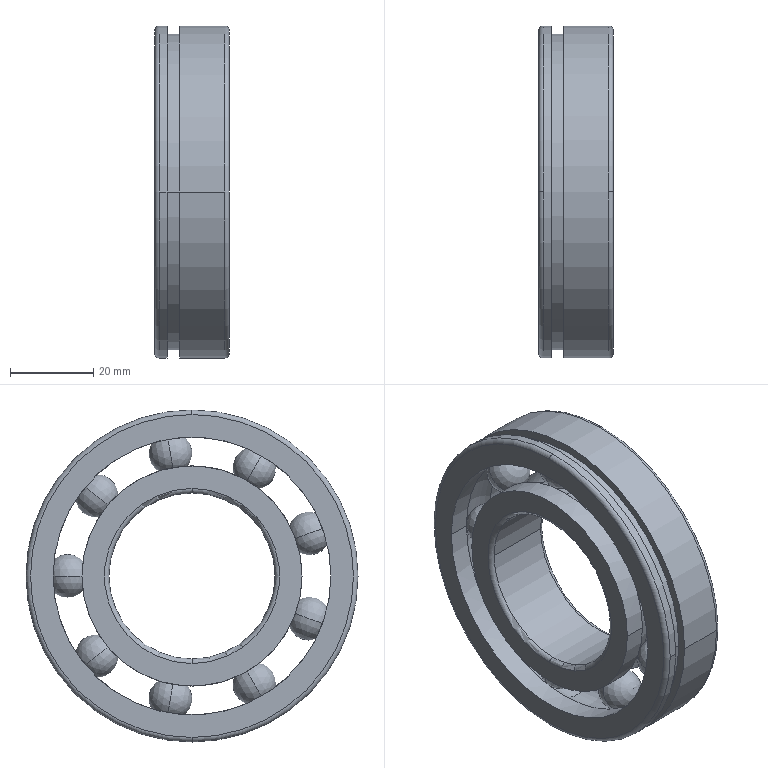Part | SolidWorks | features BaseBody 11 | 11 solids | 54 faces | box 18 x 80 x 80 mm | volume 44423 mm3 | sphere 18 | cylinder 16 | torus 14 | plane 6 | commonest cylinder face diameters 53.04 x4 66.96 x4 80 x4 40 x2 76.04 x2
STEP:
#1=CARTESIAN_POINT('',(9.,24.8,0.));
#2=VERTEX_POINT('',#1);
#3=CARTESIAN_POINT('',(9.,35.2,0.));
#4=VERTEX_POINT('',#3);
#5=CARTESIAN_POINT('',(9.,30.,0.));
#6=DIRECTION('',(0.,0.,1.));
#7=DIRECTION('',(1.,0.,0.));
#8=AXIS2_PLACEMENT_3D('',#5,#6,#7);
#9=CIRCLE('',#8,5.2);
#10=EDGE_CURVE('',#2,#4,#9,.T.);
#11=ORIENTED_EDGE('',*,*,#10,.F.);
#12=CARTESIAN_POINT('',(9.,30.,0.));
#13=DIRECTION('',(0.,0.,-1.));
#14=DIRECTION('',(-1.,0.,0.));
#15=AXIS2_PLACEMENT_3D('',#12,#13,#14);
#16=CIRCLE('',#15,5.2);
#17=EDGE_CURVE('',#2,#4,#16,.T.);
#18=ORIENTED_EDGE('',*,*,#17,.T.);
#19=EDGE_LOOP('',(#11,#18));
#20=FACE_OUTER_BOUND('',#19,.T.);
#21=CARTESIAN_POINT('',(9.,30.,0.));
#22=DIRECTION('',(0.,0.,-1.));
#23=DIRECTION('',(1.,0.,0.));
#24=AXIS2_PLACEMENT_3D('',#21,#22,#23);
#25=SPHERICAL_SURFACE('',#24,5.2);
#26=ADVANCED_FACE('',(#20),#25,.T.);
#27=ORIENTED_EDGE('',*,*,#17,.F.);
#28=ORIENTED_EDGE('',*,*,#10,.T.);
#29=EDGE_LOOP('',(#27,#28));
#30=FACE_OUTER_BOUND('',#29,.T.);
#31=CARTESIAN_POINT('',(9.,30.,0.));
#32=DIRECTION('',(0.,0.,-1.));
#33=DIRECTION('',(1.,0.,0.));
#34=AXIS2_PLACEMENT_3D('',#31,#32,#33);
#35=SPHERICAL_SURFACE('',#34,5.2);
#36=ADVANCED_FACE('',(#30),#35,.T.);
#37=CLOSED_SHELL('',(#26,#36));
#38=MANIFOLD_SOLID_BREP('',#37);
#39=CARTESIAN_POINT('',(6.,-38.02,0.));
#40=VERTEX_POINT('',#39);
#41=CARTESIAN_POINT('',(6.,38.02,0.));
#42=VERTEX_POINT('',#41);
#43=CARTESIAN_POINT('',(6.,0.,0.));
#44=DIRECTION('',(1.,0.,0.));
#45=DIRECTION('',(0.,1.,0.));
#46=AXIS2_PLACEMENT_3D('',#43,#44,#45);
#47=CIRCLE('',#46,38.02);
#48=EDGE_CURVE('',#40,#42,#47,.T.);
#49=ORIENTED_EDGE('',*,*,#48,.F.);
#50=CARTESIAN_POINT('',(3.,-38.02,0.));
#51=VERTEX_POINT('',#50);
#52=CARTESIAN_POINT('',(4.5,-38.02,0.));
#53=DIRECTION('',(-1.,0.,0.));
#54=VECTOR('',#53,1000.);
#55=LINE('',#52,#54);
#56=EDGE_CURVE('',#40,#51,#55,.T.);
#57=ORIENTED_EDGE('',*,*,#56,.T.);
#58=CARTESIAN_POINT('',(3.,38.02,0.));
#59=VERTEX_POINT('',#58);
#60=CARTESIAN_POINT('',(3.,0.,0.));
#61=DIRECTION('',(1.,0.,0.));
#62=DIRECTION('',(0.,1.,0.));
#63=AXIS2_PLACEMENT_3D('',#60,#61,#62);
#64=CIRCLE('',#63,38.02);
#65=EDGE_CURVE('',#51,#59,#64,.T.);
#66=ORIENTED_EDGE('',*,*,#65,.T.);
#67=CARTESIAN_POINT('',(4.5,38.02,0.));
#68=DIRECTION('',(-1.,0.,0.));
#69=VECTOR('',#68,1000.);
#70=LINE('',#67,#69);
#71=EDGE_CURVE('',#42,#59,#70,.T.);
#72=ORIENTED_EDGE('',*,*,#71,.F.);
#73=EDGE_LOOP('',(#49,#57,#66,#72));
#74=FACE_OUTER_BOUND('',#73,.T.);
#75=CARTESIAN_POINT('',(4.5,0.,0.));
#76=DIRECTION('',(-1.,0.,0.));
#77=DIRECTION('',(0.,1.,0.));
#78=AXIS2_PLACEMENT_3D('',#75,#76,#77);
#79=CYLINDRICAL_SURFACE('',#78,38.02);
#80=ADVANCED_FACE('',(#74),#79,.T.);
#81=CARTESIAN_POINT('',(16.9,-40.,0.));
#82=VERTEX_POINT('',#81);
#83=CARTESIAN_POINT('',(16.9,0.,-40.));
#84=VERTEX_POINT('',#83);
#85=CARTESIAN_POINT('',(16.9,0.,0.));
#86=DIRECTION('',(1.,0.,0.));
#87=DIRECTION('',(0.,-1.,0.));
#88=AXIS2_PLACEMENT_3D('',#85,#86,#87);
#89=CIRCLE('',#88,40.);
#90=EDGE_CURVE('',#82,#84,#89,.T.);
#91=ORIENTED_EDGE('',*,*,#90,.F.);
#92=CARTESIAN_POINT('',(6.,-40.,0.));
#93=VERTEX_POINT('',#92);
#94=CARTESIAN_POINT('',(12.,-40.,0.));
#95=DIRECTION('',(-1.,0.,0.));
#96=VECTOR('',#95,1000.);
#97=LINE('',#94,#96);
#98=EDGE_CURVE('',#82,#93,#97,.T.);
#99=ORIENTED_EDGE('',*,*,#98,.T.);
#100=CARTESIAN_POINT('',(6.,40.,0.));
#101=VERTEX_POINT('',#100);
#102=CARTESIAN_POINT('',(6.,0.,0.));
#103=DIRECTION('',(1.,0.,0.));
#104=DIRECTION('',(0.,1.,0.));
#105=AXIS2_PLACEMENT_3D('',#102,#103,#104);
#106=CIRCLE('',#105,40.);
#107=EDGE_CURVE('',#93,#101,#106,.T.);
#108=ORIENTED_EDGE('',*,*,#107,.T.);
#109=CARTESIAN_POINT('',(16.9,40.,0.));
#110=VERTEX_POINT('',#109);
#111=CARTESIAN_POINT('',(12.,40.,0.));
#112=DIRECTION('',(-1.,0.,0.));
#113=VECTOR('',#112,1000.);
#114=LINE('',#111,#113);
#115=EDGE_CURVE('',#110,#101,#114,.T.);
#116=ORIENTED_EDGE('',*,*,#115,.F.);
#117=CARTESIAN_POINT('',(16.9,0.,0.));
#118=DIRECTION('',(1.,0.,0.));
#119=DIRECTION('',(0.,-1.,0.));
#120=AXIS2_PLACEMENT_3D('',#117,#118,#119);
#121=CIRCLE('',#120,40.);
#122=EDGE_CURVE('',#84,#110,#121,.T.);
#123=ORIENTED_EDGE('',*,*,#122,.F.);
#124=EDGE_LOOP('',(#91,#99,#108,#116,#123));
#125=FACE_OUTER_BOUND('',#124,.T.);
#126=CARTESIAN_POINT('',(12.,0.,0.));
#127=DIRECTION('',(-1.,0.,0.));
#128=DIRECTION('',(0.,1.,0.));
#129=AXIS2_PLACEMENT_3D('',#126,#127,#128);
#130=CYLINDRICAL_SURFACE('',#129,40.);
#131=ADVANCED_FACE('',(#125),#130,.T.);
#132=CARTESIAN_POINT('',(3.,-40.,0.));
#133=VERTEX_POINT('',#132);
#134=CARTESIAN_POINT('',(3.,40.,0.));
#135=VERTEX_POINT('',#134);
#136=CARTESIAN_POINT('',(3.,0.,0.));
#137=DIRECTION('',(1.,0.,0.));
#138=DIRECTION('',(0.,1.,0.));
#139=AXIS2_PLACEMENT_3D('',#136,#137,#138);
#140=CIRCLE('',#139,40.);
#141=EDGE_CURVE('',#133,#135,#140,.T.);
#142=ORIENTED_EDGE('',*,*,#141,.F.);
#143=CARTESIAN_POINT('',(1.1,-40.,0.));
#144=VERTEX_POINT('',#143);
#145=CARTESIAN_POINT('',(1.5,-40.,0.));
#146=DIRECTION('',(-1.,0.,0.));
#147=VECTOR('',#146,1000.);
#148=LINE('',#145,#147);
#149=EDGE_CURVE('',#133,#144,#148,.T.);
#150=ORIENTED_EDGE('',*,*,#149,.T.);
#151=CARTESIAN_POINT('',(1.1,0.,-40.));
#152=VERTEX_POINT('',#151);
#153=CARTESIAN_POINT('',(1.1,0.,0.));
#154=DIRECTION('',(-1.,0.,0.));
#155=DIRECTION('',(0.,-1.,0.));
#156=AXIS2_PLACEMENT_3D('',#153,#154,#155);
#157=CIRCLE('',#156,40.);
#158=EDGE_CURVE('',#152,#144,#157,.T.);
#159=ORIENTED_EDGE('',*,*,#158,.F.);
#160=CARTESIAN_POINT('',(1.1,40.,0.));
#161=VERTEX_POINT('',#160);
#162=CARTESIAN_POINT('',(1.1,0.,0.));
#163=DIRECTION('',(-1.,0.,0.));
#164=DIRECTION('',(0.,-1.,0.));
#165=AXIS2_PLACEMENT_3D('',#162,#163,#164);
#166=CIRCLE('',#165,40.);
#167=EDGE_CURVE('',#161,#152,#166,.T.);
#168=ORIENTED_EDGE('',*,*,#167,.F.);
#169=CARTESIAN_POINT('',(1.5,40.,0.));
#170=DIRECTION('',(-1.,0.,0.));
#171=VECTOR('',#170,1000.);
#172=LINE('',#169,#171);
#173=EDGE_CURVE('',#135,#161,#172,.T.);
#174=ORIENTED_EDGE('',*,*,#173,.F.);
#175=EDGE_LOOP('',(#142,#150,#159,#168,#174));
#176=FACE_OUTER_BOUND('',#175,.T.);
#177=CARTESIAN_POINT('',(1.5,0.,0.));
#178=DIRECTION('',(-1.,0.,0.));
#179=DIRECTION('',(0.,1.,0.));
#180=AXIS2_PLACEMENT_3D('',#177,#178,#179);
#181=CYLINDRICAL_SURFACE('',#180,40.);
#182=ADVANCED_FACE('',(#176),#181,.T.);
#183=ORIENTED_EDGE('',*,*,#122,.T.);
#184=CARTESIAN_POINT('',(16.9,0.,40.));
#185=VERTEX_POINT('',#184);
#186=CARTESIAN_POINT('',(16.9,0.,0.));
#187=DIRECTION('',(1.,0.,0.));
#188=DIRECTION('',(0.,-1.,0.));
#189=AXIS2_PLACEMENT_3D('',#186,#187,#188);
#190=CIRCLE('',#189,40.);
#191=EDGE_CURVE('',#110,#185,#190,.T.);
#192=ORIENTED_EDGE('',*,*,#191,.T.);
#193=CARTESIAN_POINT('',(18.,0.,38.9));
#194=VERTEX_POINT('',#193);
#195=CARTESIAN_POINT('',(16.9,0.,38.9));
#196=DIRECTION('',(0.,1.,0.));
#197=DIRECTION('',(0.,0.,1.));
#198=AXIS2_PLACEMENT_3D('',#195,#196,#197);
#199=CIRCLE('',#198,1.1);
#200=EDGE_CURVE('',#185,#194,#199,.T.);
#201=ORIENTED_EDGE('',*,*,#200,.T.);
#202=CARTESIAN_POINT('',(18.,0.,-38.9));
#203=VERTEX_POINT('',#202);
#204=CARTESIAN_POINT('',(18.,0.,0.));
#205=DIRECTION('',(-1.,0.,0.));
#206=DIRECTION('',(0.,-1.,0.));
#207=AXIS2_PLACEMENT_3D('',#204,#205,#206);
#208=CIRCLE('',#207,38.9);
#209=EDGE_CURVE('',#194,#203,#208,.T.);
#210=ORIENTED_EDGE('',*,*,#209,.T.);
#211=CARTESIAN_POINT('',(16.9,0.,-38.9));
#212=DIRECTION('',(0.,-1.,0.));
#213=DIRECTION('',(0.,0.,-1.));
#214=AXIS2_PLACEMENT_3D('',#211,#212,#213);
#215=CIRCLE('',#214,1.1);
#216=EDGE_CURVE('',#84,#203,#215,.T.);
#217=ORIENTED_EDGE('',*,*,#216,.F.);
#218=EDGE_LOOP('',(#183,#192,#201,#210,#217));
#219=FACE_OUTER_BOUND('',#218,.T.);
#220=CARTESIAN_POINT('',(16.9,0.,0.));
#221=DIRECTION('',(1.,0.,0.));
#222=DIRECTION('',(0.,0.,-1.));
#223=AXIS2_PLACEMENT_3D('',#220,#221,#222);
#224=TOROIDAL_SURFACE('',#223,38.9,1.1);
#225=ADVANCED_FACE('',(#219),#224,.T.);
#226=CARTESIAN_POINT('',(0.,0.,-38.9));
#227=VERTEX_POINT('',#226);
#228=CARTESIAN_POINT('',(0.,0.,38.9));
#229=VERTEX_POINT('',#228);
#230=CARTESIAN_POINT('',(0.,0.,0.));
#231=DIRECTION('',(1.,0.,0.));
#232=DIRECTION('',(0.,-1.,0.));
#233=AXIS2_PLACEMENT_3D('',#230,#231,#232);
#234=CIRCLE('',#233,38.9);
#235=EDGE_CURVE('',#227,#229,#234,.T.);
#236=ORIENTED_EDGE('',*,*,#235,.T.);
#237=CARTESIAN_POINT('',(1.1,0.,40.));
#238=VERTEX_POINT('',#237);
#239=CARTESIAN_POINT('',(1.1,0.,38.9));
#240=DIRECTION('',(0.,1.,0.));
#241=DIRECTION('',(0.,0.,1.));
#242=AXIS2_PLACEMENT_3D('',#239,#240,#241);
#243=CIRCLE('',#242,1.1);
#244=EDGE_CURVE('',#229,#238,#243,.T.);
#245=ORIENTED_EDGE('',*,*,#244,.T.);
#246=CARTESIAN_POINT('',(1.1,0.,0.));
#247=DIRECTION('',(-1.,0.,0.));
#248=DIRECTION('',(0.,-1.,0.));
#249=AXIS2_PLACEMENT_3D('',#246,#247,#248);
#250=CIRCLE('',#249,40.);
#251=EDGE_CURVE('',#238,#161,#250,.T.);
#252=ORIENTED_EDGE('',*,*,#251,.T.);
#253=ORIENTED_EDGE('',*,*,#167,.T.);
#254=CARTESIAN_POINT('',(1.1,0.,-38.9));
#255=DIRECTION('',(0.,-1.,0.));
#256=DIRECTION('',(0.,0.,-1.));
#257=AXIS2_PLACEMENT_3D('',#254,#255,#256);
#258=CIRCLE('',#257,1.1);
#259=EDGE_CURVE('',#227,#152,#258,.T.);
#260=ORIENTED_EDGE('',*,*,#259,.F.);
#261=EDGE_LOOP('',(#236,#245,#252,#253,#260));
#262=FACE_OUTER_BOUND('',#261,.T.);
#263=CARTESIAN_POINT('',(1.1,0.,0.));
#264=DIRECTION('',(1.,0.,0.));
#265=DIRECTION('',(0.,0.,-1.));
#266=AXIS2_PLACEMENT_3D('',#263,#264,#265);
#267=TOROIDAL_SURFACE('',#266,38.9,1.1);
#268=ADVANCED_FACE('',(#262),#267,.T.);
#269=CARTESIAN_POINT('',(5.136,0.,33.48));
#270=VERTEX_POINT('',#269);
#271=CARTESIAN_POINT('',(5.136,-33.48,0.));
#272=VERTEX_POINT('',#271);
#273=CARTESIAN_POINT('',(5.136,0.,0.));
#274=DIRECTION('',(1.,0.,0.));
#275=DIRECTION('',(0.,1.,0.));
#276=AXIS2_PLACEMENT_3D('',#273,#274,#275);
#277=CIRCLE('',#276,33.48);
#278=EDGE_CURVE('',#270,#272,#277,.T.);
#279=ORIENTED_EDGE('',*,*,#278,.F.);
#280=CARTESIAN_POINT('',(12.864,0.,33.48));
#281=VERTEX_POINT('',#280);
#282=CARTESIAN_POINT('',(9.,0.,30.));
#283=DIRECTION('',(0.,1.,0.));
#284=DIRECTION('',(0.,0.,1.));
#285=AXIS2_PLACEMENT_3D('',#282,#283,#284);
#286=CIRCLE('',#285,5.2);
#287=EDGE_CURVE('',#270,#281,#286,.T.);
#288=ORIENTED_EDGE('',*,*,#287,.T.);
#289=CARTESIAN_POINT('',(12.864,-33.48,0.));
#290=VERTEX_POINT('',#289);
#291=CARTESIAN_POINT('',(12.864,0.,0.));
#292=DIRECTION('',(1.,0.,0.));
#293=DIRECTION('',(0.,1.,0.));
#294=AXIS2_PLACEMENT_3D('',#291,#292,#293);
#295=CIRCLE('',#294,33.48);
#296=EDGE_CURVE('',#281,#290,#295,.T.);
#297=ORIENTED_EDGE('',*,*,#296,.T.);
#298=CARTESIAN_POINT('',(12.864,0.,-33.48));
#299=VERTEX_POINT('',#298);
#300=CARTESIAN_POINT('',(12.864,0.,0.));
#301=DIRECTION('',(1.,0.,0.));
#302=DIRECTION('',(0.,1.,0.));
#303=AXIS2_PLACEMENT_3D('',#300,#301,#302);
#304=CIRCLE('',#303,33.48);
#305=EDGE_CURVE('',#290,#299,#304,.T.);
#306=ORIENTED_EDGE('',*,*,#305,.T.);
#307=CARTESIAN_POINT('',(5.136,0.,-33.48));
#308=VERTEX_POINT('',#307);
#309=CARTESIAN_POINT('',(9.,0.,-30.));
#310=DIRECTION('',(0.,-1.,0.));
#311=DIRECTION('',(0.,0.,-1.));
#312=AXIS2_PLACEMENT_3D('',#309,#310,#311);
#313=CIRCLE('',#312,5.2);
#314=EDGE_CURVE('',#308,#299,#313,.T.);
#315=ORIENTED_EDGE('',*,*,#314,.F.);
#316=CARTESIAN_POINT('',(5.136,0.,0.));
#317=DIRECTION('',(1.,0.,0.));
#318=DIRECTION('',(0.,1.,0.));
#319=AXIS2_PLACEMENT_3D('',#316,#317,#318);
#320=CIRCLE('',#319,33.48);
#321=EDGE_CURVE('',#272,#308,#320,.T.);
#322=ORIENTED_EDGE('',*,*,#321,.F.);
#323=EDGE_LOOP('',(#279,#288,#297,#306,#315,#322));
#324=FACE_OUTER_BOUND('',#323,.T.);
#325=CARTESIAN_POINT('',(9.,0.,0.));
#326=DIRECTION('',(1.,0.,0.));
#327=DIRECTION('',(0.,0.,-1.));
#328=AXIS2_PLACEMENT_3D('',#325,#326,#327);
#329=TOROIDAL_SURFACE('',#328,30.,5.2);
#330=ADVANCED_FACE('',(#324),#329,.F.);
#331=CARTESIAN_POINT('',(18.,33.48,0.));
#332=VERTEX_POINT('',#331);
#333=CARTESIAN_POINT('',(18.,-33.48,0.));
#334=VERTEX_POINT('',#333);
#335=CARTESIAN_POINT('',(18.,0.,0.));
#336=DIRECTION('',(1.,0.,0.));
#337=DIRECTION('',(0.,1.,0.));
#338=AXIS2_PLACEMENT_3D('',#335,#336,#337);
#339=CIRCLE('',#338,33.48);
#340=EDGE_CURVE('',#332,#334,#339,.T.);
#341=ORIENTED_EDGE('',*,*,#340,.T.);
#342=CARTESIAN_POINT('',(15.432,-33.48,0.));
#343=DIRECTION('',(-1.,0.,0.));
#344=VECTOR('',#343,1000.);
#345=LINE('',#342,#344);
#346=EDGE_CURVE('',#334,#290,#345,.T.);
#347=ORIENTED_EDGE('',*,*,#346,.T.);
#348=ORIENTED_EDGE('',*,*,#296,.F.);
#349=CARTESIAN_POINT('',(12.864,33.48,0.));
#350=VERTEX_POINT('',#349);
#351=CARTESIAN_POINT('',(12.864,0.,0.));
#352=DIRECTION('',(1.,0.,0.));
#353=DIRECTION('',(0.,1.,0.));
#354=AXIS2_PLACEMENT_3D('',#351,#352,#353);
#355=CIRCLE('',#354,33.48);
#356=EDGE_CURVE('',#350,#281,#355,.T.);
#357=ORIENTED_EDGE('',*,*,#356,.F.);
#358=CARTESIAN_POINT('',(15.432,33.48,0.));
#359=DIRECTION('',(-1.,0.,0.));
#360=VECTOR('',#359,1000.);
#361=LINE('',#358,#360);
#362=EDGE_CURVE('',#332,#350,#361,.T.);
#363=ORIENTED_EDGE('',*,*,#362,.F.);
#364=EDGE_LOOP('',(#341,#347,#348,#357,#363));
#365=FACE_OUTER_BOUND('',#364,.T.);
#366=CARTESIAN_POINT('',(15.432,0.,0.));
#367=DIRECTION('',(-1.,0.,0.));
#368=DIRECTION('',(0.,1.,0.));
#369=AXIS2_PLACEMENT_3D('',#366,#367,#368);
#370=CYLINDRICAL_SURFACE('',#369,33.48);
#371=ADVANCED_FACE('',(#365),#370,.F.);
#372=CARTESIAN_POINT('',(5.136,33.48,0.));
#373=VERTEX_POINT('',#372);
#374=CARTESIAN_POINT('',(5.136,0.,0.));
#375=DIRECTION('',(1.,0.,0.));
#376=DIRECTION('',(0.,1.,0.));
#377=AXIS2_PLACEMENT_3D('',#374,#375,#376);
#378=CIRCLE('',#377,33.48);
#379=EDGE_CURVE('',#373,#270,#378,.T.);
#380=ORIENTED_EDGE('',*,*,#379,.T.);
#381=ORIENTED_EDGE('',*,*,#278,.T.);
#382=CARTESIAN_POINT('',(0.,-33.48,0.));
#383=VERTEX_POINT('',#382);
#384=CARTESIAN_POINT('',(2.568,-33.48,0.));
#385=DIRECTION('',(-1.,0.,0.));
#386=VECTOR('',#385,1000.);
#387=LINE('',#384,#386);
#388=EDGE_CURVE('',#272,#383,#387,.T.);
#389=ORIENTED_EDGE('',*,*,#388,.T.);
#390=CARTESIAN_POINT('',(0.,33.48,0.));
#391=VERTEX_POINT('',#390);
#392=CARTESIAN_POINT('',(0.,0.,0.));
#393=DIRECTION('',(1.,0.,0.));
#394=DIRECTION('',(0.,1.,0.));
#395=AXIS2_PLACEMENT_3D('',#392,#393,#394);
#396=CIRCLE('',#395,33.48);
#397=EDGE_CURVE('',#391,#383,#396,.T.);
#398=ORIENTED_EDGE('',*,*,#397,.F.);
#399=CARTESIAN_POINT('',(2.568,33.48,0.));
#400=DIRECTION('',(-1.,0.,0.));
#401=VECTOR('',#400,1000.);
#402=LINE('',#399,#401);
#403=EDGE_CURVE('',#373,#391,#402,.T.);
#404=ORIENTED_EDGE('',*,*,#403,.F.);
#405=EDGE_LOOP('',(#380,#381,#389,#398,#404));
#406=FACE_OUTER_BOUND('',#405,.T.);
#407=CARTESIAN_POINT('',(2.568,0.,0.));
#408=DIRECTION('',(-1.,0.,0.));
#409=DIRECTION('',(0.,1.,0.));
#410=AXIS2_PLACEMENT_3D('',#407,#408,#409);
#411=CYLINDRICAL_SURFACE('',#410,33.48);
#412=ADVANCED_FACE('',(#406),#411,.F.);
#413=CARTESIAN_POINT('',(6.,0.,0.));
#414=DIRECTION('',(1.,0.,0.));
#415=DIRECTION('',(0.,1.,0.));
#416=AXIS2_PLACEMENT_3D('',#413,#414,#415);
#417=CIRCLE('',#416,38.02);
#418=EDGE_CURVE('',#42,#40,#417,.T.);
#419=ORIENTED_EDGE('',*,*,#418,.T.);
#420=ORIENTED_EDGE('',*,*,#48,.T.);
#421=EDGE_LOOP('',(#419,#420));
#422=FACE_BOUND('',#421,.T.);
#423=CARTESIAN_POINT('',(6.,0.,0.));
#424=DIRECTION('',(1.,0.,0.));
#425=DIRECTION('',(0.,1.,0.));
#426=AXIS2_PLACEMENT_3D('',#423,#424,#425);
#427=CIRCLE('',#426,40.);
#428=EDGE_CURVE('',#101,#93,#427,.T.);
#429=ORIENTED_EDGE('',*,*,#428,.F.);
#430=ORIENTED_EDGE('',*,*,#107,.F.);
#431=EDGE_LOOP('',(#429,#430));
#432=FACE_OUTER_BOUND('',#431,.T.);
#433=CARTESIAN_POINT('',(6.,39.01,0.));
#434=DIRECTION('',(-1.,0.,0.));
#435=DIRECTION('',(0.,0.,1.));
#436=AXIS2_PLACEMENT_3D('',#433,#434,#435);
#437=PLANE('',#436);
#438=ADVANCED_FACE('',(#422,#432),#437,.T.);
#439=CARTESIAN_POINT('',(3.,0.,0.));
#440=DIRECTION('',(1.,0.,0.));
#441=DIRECTION('',(0.,1.,0.));
#442=AXIS2_PLACEMENT_3D('',#439,#440,#441);
#443=CIRCLE('',#442,38.02);
#444=EDGE_CURVE('',#59,#51,#443,.T.);
#445=ORIENTED_EDGE('',*,*,#444,.F.);
#446=ORIENTED_EDGE('',*,*,#65,.F.);
#447=EDGE_LOOP('',(#445,#446));
#448=FACE_BOUND('',#447,.T.);
#449=CARTESIAN_POINT('',(3.,0.,0.));
#450=DIRECTION('',(1.,0.,0.));
#451=DIRECTION('',(0.,1.,0.));
#452=AXIS2_PLACEMENT_3D('',#449,#450,#451);
#453=CIRCLE('',#452,40.);
#454=EDGE_CURVE('',#135,#133,#453,.T.);
#455=ORIENTED_EDGE('',*,*,#454,.T.);
#456=ORIENTED_EDGE('',*,*,#141,.T.);
#457=EDGE_LOOP('',(#455,#456));
#458=FACE_OUTER_BOUND('',#457,.T.);
#459=CARTESIAN_POINT('',(3.,39.01,0.));
#460=DIRECTION('',(1.,0.,0.));
#461=DIRECTION('',(0.,1.,0.));
#462=AXIS2_PLACEMENT_3D('',#459,#460,#461);
#463=PLANE('',#462);
#464=ADVANCED_FACE('',(#448,#458),#463,.T.);
#465=ORIENTED_EDGE('',*,*,#340,.F.);
#466=CARTESIAN_POINT('',(18.,0.,0.));
#467=DIRECTION('',(1.,0.,0.));
#468=DIRECTION('',(0.,1.,0.));
#469=AXIS2_PLACEMENT_3D('',#466,#467,#468);
#470=CIRCLE('',#469,33.48);
#471=EDGE_CURVE('',#334,#332,#470,.T.);
#472=ORIENTED_EDGE('',*,*,#471,.F.);
#473=EDGE_LOOP('',(#465,#472));
#474=FACE_BOUND('',#473,.T.);
#475=CARTESIAN_POINT('',(18.,0.,0.));
#476=DIRECTION('',(-1.,0.,0.));
#477=DIRECTION('',(0.,-1.,0.));
#478=AXIS2_PLACEMENT_3D('',#475,#476,#477);
#479=CIRCLE('',#478,38.9);
#480=EDGE_CURVE('',#203,#194,#479,.T.);
#481=ORIENTED_EDGE('',*,*,#480,.F.);
#482=ORIENTED_EDGE('',*,*,#209,.F.);
#483=EDGE_LOOP('',(#481,#482));
#484=FACE_OUTER_BOUND('',#483,.T.);
#485=CARTESIAN_POINT('',(18.,36.74,0.));
#486=DIRECTION('',(1.,0.,0.));
#487=DIRECTION('',(0.,1.,0.));
#488=AXIS2_PLACEMENT_3D('',#485,#486,#487);
#489=PLANE('',#488);
#490=ADVANCED_FACE('',(#474,#484),#489,.T.);
#491=ORIENTED_EDGE('',*,*,#397,.T.);
#492=CARTESIAN_POINT('',(0.,0.,0.));
#493=DIRECTION('',(1.,0.,0.));
#494=DIRECTION('',(0.,1.,0.));
#495=AXIS2_PLACEMENT_3D('',#492,#493,#494);
#496=CIRCLE('',#495,33.48);
#497=EDGE_CURVE('',#383,#391,#496,.T.);
#498=ORIENTED_EDGE('',*,*,#497,.T.);
#499=EDGE_LOOP('',(#491,#498));
#500=FACE_BOUND('',#499,.T.);
#501=ORIENTED_EDGE('',*,*,#235,.F.);
#502=CARTESIAN_POINT('',(0.,0.,0.));
#503=DIRECTION('',(1.,0.,0.));
#504=DIRECTION('',(0.,-1.,0.));
#505=AXIS2_PLACEMENT_3D('',#502,#503,#504);
#506=CIRCLE('',#505,38.9);
#507=EDGE_CURVE('',#229,#227,#506,.T.);
#508=ORIENTED_EDGE('',*,*,#507,.F.);
#509=EDGE_LOOP('',(#501,#508));
#510=FACE_OUTER_BOUND('',#509,.T.);
#511=CARTESIAN_POINT('',(0.,36.74,0.));
#512=DIRECTION('',(-1.,0.,0.));
#513=DIRECTION('',(0.,0.,1.));
#514=AXIS2_PLACEMENT_3D('',#511,#512,#513);
#515=PLANE('',#514);
#516=ADVANCED_FACE('',(#500,#510),#515,.T.);
#517=ORIENTED_EDGE('',*,*,#388,.F.);
#518=ORIENTED_EDGE('',*,*,#321,.T.);
#519=CARTESIAN_POINT('',(5.136,0.,0.));
#520=DIRECTION('',(1.,0.,0.));
#521=DIRECTION('',(0.,1.,0.));
#522=AXIS2_PLACEMENT_3D('',#519,#520,#521);
#523=CIRCLE('',#522,33.48);
#524=EDGE_CURVE('',#308,#373,#523,.T.);
#525=ORIENTED_EDGE('',*,*,#524,.T.);
#526=ORIENTED_EDGE('',*,*,#403,.T.);
#527=ORIENTED_EDGE('',*,*,#497,.F.);
#528=EDGE_LOOP('',(#517,#518,#525,#526,#527));
#529=FACE_OUTER_BOUND('',#528,.T.);
#530=CARTESIAN_POINT('',(2.568,0.,0.));
#531=DIRECTION('',(-1.,0.,0.));
#532=DIRECTION('',(0.,1.,0.));
#533=AXIS2_PLACEMENT_3D('',#530,#531,#532);
#534=CYLINDRICAL_SURFACE('',#533,33.48);
#535=ADVANCED_FACE('',(#529),#534,.F.);
#536=ORIENTED_EDGE('',*,*,#346,.F.);
#537=ORIENTED_EDGE('',*,*,#471,.T.);
#538=ORIENTED_EDGE('',*,*,#362,.T.);
#539=CARTESIAN_POINT('',(12.864,0.,0.));
#540=DIRECTION('',(1.,0.,0.));
#541=DIRECTION('',(0.,1.,0.));
#542=AXIS2_PLACEMENT_3D('',#539,#540,#541);
#543=CIRCLE('',#542,33.48);
#544=EDGE_CURVE('',#299,#350,#543,.T.);
#545=ORIENTED_EDGE('',*,*,#544,.F.);
#546=ORIENTED_EDGE('',*,*,#305,.F.);
#547=EDGE_LOOP('',(#536,#537,#538,#545,#546));
#548=FACE_OUTER_BOUND('',#547,.T.);
#549=CARTESIAN_POINT('',(15.432,0.,0.));
#550=DIRECTION('',(-1.,0.,0.));
#551=DIRECTION('',(0.,1.,0.));
#552=AXIS2_PLACEMENT_3D('',#549,#550,#551);
#553=CYLINDRICAL_SURFACE('',#552,33.48);
#554=ADVANCED_FACE('',(#548),#553,.F.);
#555=ORIENTED_EDGE('',*,*,#287,.F.);
#556=ORIENTED_EDGE('',*,*,#379,.F.);
#557=ORIENTED_EDGE('',*,*,#524,.F.);
#558=ORIENTED_EDGE('',*,*,#314,.T.);
#559=ORIENTED_EDGE('',*,*,#544,.T.);
#560=ORIENTED_EDGE('',*,*,#356,.T.);
#561=EDGE_LOOP('',(#555,#556,#557,#558,#559,#560));
#562=FACE_OUTER_BOUND('',#561,.T.);
#563=CARTESIAN_POINT('',(9.,0.,0.));
#564=DIRECTION('',(1.,0.,0.));
#565=DIRECTION('',(0.,0.,-1.));
#566=AXIS2_PLACEMENT_3D('',#563,#564,#565);
#567=TOROIDAL_SURFACE('',#566,30.,5.2);
#568=ADVANCED_FACE('',(#562),#567,.F.);
#569=ORIENTED_EDGE('',*,*,#244,.F.);
#570=ORIENTED_EDGE('',*,*,#507,.T.);
#571=ORIENTED_EDGE('',*,*,#259,.T.);
#572=ORIENTED_EDGE('',*,*,#158,.T.);
#573=CARTESIAN_POINT('',(1.1,0.,0.));
#574=DIRECTION('',(-1.,0.,0.));
#575=DIRECTION('',(0.,-1.,0.));
#576=AXIS2_PLACEMENT_3D('',#573,#574,#575);
#577=CIRCLE('',#576,40.);
#578=EDGE_CURVE('',#144,#238,#577,.T.);
#579=ORIENTED_EDGE('',*,*,#578,.T.);
#580=EDGE_LOOP('',(#569,#570,#571,#572,#579));
#581=FACE_OUTER_BOUND('',#580,.T.);
#582=CARTESIAN_POINT('',(1.1,0.,0.));
#583=DIRECTION('',(1.,0.,0.));
#584=DIRECTION('',(0.,0.,-1.));
#585=AXIS2_PLACEMENT_3D('',#582,#583,#584);
#586=TOROIDAL_SURFACE('',#585,38.9,1.1);
#587=ADVANCED_FACE('',(#581),#586,.T.);
#588=ORIENTED_EDGE('',*,*,#200,.F.);
#589=CARTESIAN_POINT('',(16.9,0.,0.));
#590=DIRECTION('',(1.,0.,0.));
#591=DIRECTION('',(0.,-1.,0.));
#592=AXIS2_PLACEMENT_3D('',#589,#590,#591);
#593=CIRCLE('',#592,40.);
#594=EDGE_CURVE('',#185,#82,#593,.T.);
#595=ORIENTED_EDGE('',*,*,#594,.T.);
#596=ORIENTED_EDGE('',*,*,#90,.T.);
#597=ORIENTED_EDGE('',*,*,#216,.T.);
#598=ORIENTED_EDGE('',*,*,#480,.T.);
#599=EDGE_LOOP('',(#588,#595,#596,#597,#598));
#600=FACE_OUTER_BOUND('',#599,.T.);
#601=CARTESIAN_POINT('',(16.9,0.,0.));
#602=DIRECTION('',(1.,0.,0.));
#603=DIRECTION('',(0.,0.,-1.));
#604=AXIS2_PLACEMENT_3D('',#601,#602,#603);
#605=TOROIDAL_SURFACE('',#604,38.9,1.1);
#606=ADVANCED_FACE('',(#600),#605,.T.);
#607=ORIENTED_EDGE('',*,*,#149,.F.);
#608=ORIENTED_EDGE('',*,*,#454,.F.);
#609=ORIENTED_EDGE('',*,*,#173,.T.);
#610=ORIENTED_EDGE('',*,*,#251,.F.);
#611=ORIENTED_EDGE('',*,*,#578,.F.);
#612=EDGE_LOOP('',(#607,#608,#609,#610,#611));
#613=FACE_OUTER_BOUND('',#612,.T.);
#614=CARTESIAN_POINT('',(1.5,0.,0.));
#615=DIRECTION('',(-1.,0.,0.));
#616=DIRECTION('',(0.,1.,0.));
#617=AXIS2_PLACEMENT_3D('',#614,#615,#616);
#618=CYLINDRICAL_SURFACE('',#617,40.);
#619=ADVANCED_FACE('',(#613),#618,.T.);
#620=ORIENTED_EDGE('',*,*,#98,.F.);
#621=ORIENTED_EDGE('',*,*,#594,.F.);
#622=ORIENTED_EDGE('',*,*,#191,.F.);
#623=ORIENTED_EDGE('',*,*,#115,.T.);
#624=ORIENTED_EDGE('',*,*,#428,.T.);
#625=EDGE_LOOP('',(#620,#621,#622,#623,#624));
#626=FACE_OUTER_BOUND('',#625,.T.);
#627=CARTESIAN_POINT('',(12.,0.,0.));
#628=DIRECTION('',(-1.,0.,0.));
#629=DIRECTION('',(0.,1.,0.));
#630=AXIS2_PLACEMENT_3D('',#627,#628,#629);
#631=CYLINDRICAL_SURFACE('',#630,40.);
#632=ADVANCED_FACE('',(#626),#631,.T.);
#633=ORIENTED_EDGE('',*,*,#56,.F.);
#634=ORIENTED_EDGE('',*,*,#418,.F.);
#635=ORIENTED_EDGE('',*,*,#71,.T.);
#636=ORIENTED_EDGE('',*,*,#444,.T.);
#637=EDGE_LOOP('',(#633,#634,#635,#636));
#638=FACE_OUTER_BOUND('',#637,.T.);
#639=CARTESIAN_POINT('',(4.5,0.,0.));
#640=DIRECTION('',(-1.,0.,0.));
#641=DIRECTION('',(0.,1.,0.));
#642=AXIS2_PLACEMENT_3D('',#639,#640,#641);
#643=CYLINDRICAL_SURFACE('',#642,38.02);
#644=ADVANCED_FACE('',(#638),#643,.T.);
#645=CLOSED_SHELL('',(#80,#131,#182,#225,#268,#330,#371,#412,#438,#464,#490,#516,#535,#554,#568,#587,#606,#619,#632,#644));
#646=MANIFOLD_SOLID_BREP('',#645);
#647=CARTESIAN_POINT('',(12.864,0.,-26.52));
#648=VERTEX_POINT('',#647);
#649=CARTESIAN_POINT('',(9.,0.,-24.8));
#650=VERTEX_POINT('',#649);
#651=CARTESIAN_POINT('',(9.,0.,-30.));
#652=DIRECTION('',(0.,-1.,0.));
#653=DIRECTION('',(0.,0.,-1.));
#654=AXIS2_PLACEMENT_3D('',#651,#652,#653);
#655=CIRCLE('',#654,5.2);
#656=EDGE_CURVE('',#648,#650,#655,.T.);
#657=ORIENTED_EDGE('',*,*,#656,.T.);
#658=CARTESIAN_POINT('',(9.,0.,24.8));
#659=VERTEX_POINT('',#658);
#660=CARTESIAN_POINT('',(9.,0.,0.));
#661=DIRECTION('',(1.,0.,0.));
#662=DIRECTION('',(0.,0.,-1.));
#663=AXIS2_PLACEMENT_3D('',#660,#661,#662);
#664=CIRCLE('',#663,24.8);
#665=EDGE_CURVE('',#650,#659,#664,.T.);
#666=ORIENTED_EDGE('',*,*,#665,.T.);
#667=CARTESIAN_POINT('',(12.864,0.,26.52));
#668=VERTEX_POINT('',#667);
#669=CARTESIAN_POINT('',(9.,0.,30.));
#670=DIRECTION('',(0.,1.,0.));
#671=DIRECTION('',(0.,0.,1.));
#672=AXIS2_PLACEMENT_3D('',#669,#670,#671);
#673=CIRCLE('',#672,5.2);
#674=EDGE_CURVE('',#668,#659,#673,.T.);
#675=ORIENTED_EDGE('',*,*,#674,.F.);
#676=CARTESIAN_POINT('',(12.864,26.52,0.));
#677=VERTEX_POINT('',#676);
#678=CARTESIAN_POINT('',(12.864,0.,0.));
#679=DIRECTION('',(1.,0.,0.));
#680=DIRECTION('',(0.,1.,0.));
#681=AXIS2_PLACEMENT_3D('',#678,#679,#680);
#682=CIRCLE('',#681,26.52);
#683=EDGE_CURVE('',#677,#668,#682,.T.);
#684=ORIENTED_EDGE('',*,*,#683,.F.);
#685=CARTESIAN_POINT('',(12.864,0.,0.));
#686=DIRECTION('',(1.,0.,0.));
#687=DIRECTION('',(0.,1.,0.));
#688=AXIS2_PLACEMENT_3D('',#685,#686,#687);
#689=CIRCLE('',#688,26.52);
#690=EDGE_CURVE('',#648,#677,#689,.T.);
#691=ORIENTED_EDGE('',*,*,#690,.F.);
#692=EDGE_LOOP('',(#657,#666,#675,#684,#691));
#693=FACE_OUTER_BOUND('',#692,.T.);
#694=CARTESIAN_POINT('',(9.,0.,0.));
#695=DIRECTION('',(1.,0.,0.));
#696=DIRECTION('',(0.,0.,-1.));
#697=AXIS2_PLACEMENT_3D('',#694,#695,#696);
#698=TOROIDAL_SURFACE('',#697,30.,5.2);
#699=ADVANCED_FACE('',(#693),#698,.F.);
#700=ORIENTED_EDGE('',*,*,#674,.T.);
#701=CARTESIAN_POINT('',(9.,0.,0.));
#702=DIRECTION('',(1.,0.,0.));
#703=DIRECTION('',(0.,0.,-1.));
#704=AXIS2_PLACEMENT_3D('',#701,#702,#703);
#705=CIRCLE('',#704,24.8);
#706=EDGE_CURVE('',#659,#650,#705,.T.);
#707=ORIENTED_EDGE('',*,*,#706,.T.);
#708=ORIENTED_EDGE('',*,*,#656,.F.);
#709=CARTESIAN_POINT('',(12.864,-26.52,0.));
#710=VERTEX_POINT('',#709);
#711=CARTESIAN_POINT('',(12.864,0.,0.));
#712=DIRECTION('',(1.,0.,0.));
#713=DIRECTION('',(0.,1.,0.));
#714=AXIS2_PLACEMENT_3D('',#711,#712,#713);
#715=CIRCLE('',#714,26.52);
#716=EDGE_CURVE('',#710,#648,#715,.T.);
#717=ORIENTED_EDGE('',*,*,#716,.F.);
#718=CARTESIAN_POINT('',(12.864,0.,0.));
#719=DIRECTION('',(1.,0.,0.));
#720=DIRECTION('',(0.,1.,0.));
#721=AXIS2_PLACEMENT_3D('',#718,#719,#720);
#722=CIRCLE('',#721,26.52);
#723=EDGE_CURVE('',#668,#710,#722,.T.);
#724=ORIENTED_EDGE('',*,*,#723,.F.);
#725=EDGE_LOOP('',(#700,#707,#708,#717,#724));
#726=FACE_OUTER_BOUND('',#725,.T.);
#727=CARTESIAN_POINT('',(9.,0.,0.));
#728=DIRECTION('',(1.,0.,0.));
#729=DIRECTION('',(0.,0.,-1.));
#730=AXIS2_PLACEMENT_3D('',#727,#728,#729);
#731=TOROIDAL_SURFACE('',#730,30.,5.2);
#732=ADVANCED_FACE('',(#726),#731,.F.);
#733=ORIENTED_EDGE('',*,*,#706,.F.);
#734=CARTESIAN_POINT('',(5.136,0.,26.52));
#735=VERTEX_POINT('',#734);
#736=CARTESIAN_POINT('',(9.,0.,30.));
#737=DIRECTION('',(0.,1.,0.));
#738=DIRECTION('',(0.,0.,1.));
#739=AXIS2_PLACEMENT_3D('',#736,#737,#738);
#740=CIRCLE('',#739,5.2);
#741=EDGE_CURVE('',#659,#735,#740,.T.);
#742=ORIENTED_EDGE('',*,*,#741,.T.);
#743=CARTESIAN_POINT('',(5.136,-26.52,0.));
#744=VERTEX_POINT('',#743);
#745=CARTESIAN_POINT('',(5.136,0.,0.));
#746=DIRECTION('',(1.,0.,0.));
#747=DIRECTION('',(0.,1.,0.));
#748=AXIS2_PLACEMENT_3D('',#745,#746,#747);
#749=CIRCLE('',#748,26.52);
#750=EDGE_CURVE('',#735,#744,#749,.T.);
#751=ORIENTED_EDGE('',*,*,#750,.T.);
#752=CARTESIAN_POINT('',(5.136,0.,-26.52));
#753=VERTEX_POINT('',#752);
#754=CARTESIAN_POINT('',(5.136,0.,0.));
#755=DIRECTION('',(1.,0.,0.));
#756=DIRECTION('',(0.,1.,0.));
#757=AXIS2_PLACEMENT_3D('',#754,#755,#756);
#758=CIRCLE('',#757,26.52);
#759=EDGE_CURVE('',#744,#753,#758,.T.);
#760=ORIENTED_EDGE('',*,*,#759,.T.);
#761=CARTESIAN_POINT('',(9.,0.,-30.));
#762=DIRECTION('',(0.,-1.,0.));
#763=DIRECTION('',(0.,0.,-1.));
#764=AXIS2_PLACEMENT_3D('',#761,#762,#763);
#765=CIRCLE('',#764,5.2);
#766=EDGE_CURVE('',#650,#753,#765,.T.);
#767=ORIENTED_EDGE('',*,*,#766,.F.);
#768=EDGE_LOOP('',(#733,#742,#751,#760,#767));
#769=FACE_OUTER_BOUND('',#768,.T.);
#770=CARTESIAN_POINT('',(9.,0.,0.));
#771=DIRECTION('',(1.,0.,0.));
#772=DIRECTION('',(0.,0.,-1.));
#773=AXIS2_PLACEMENT_3D('',#770,#771,#772);
#774=TOROIDAL_SURFACE('',#773,30.,5.2);
#775=ADVANCED_FACE('',(#769),#774,.F.);
#776=CARTESIAN_POINT('',(16.9,-20.,0.));
#777=VERTEX_POINT('',#776);
#778=CARTESIAN_POINT('',(16.9,0.,20.));
#779=VERTEX_POINT('',#778);
#780=CARTESIAN_POINT('',(16.9,0.,0.));
#781=DIRECTION('',(-1.,0.,0.));
#782=DIRECTION('',(0.,-1.,0.));
#783=AXIS2_PLACEMENT_3D('',#780,#781,#782);
#784=CIRCLE('',#783,20.);
#785=EDGE_CURVE('',#777,#779,#784,.T.);
#786=ORIENTED_EDGE('',*,*,#785,.F.);
#787=CARTESIAN_POINT('',(1.1,-20.,0.));
#788=VERTEX_POINT('',#787);
#789=CARTESIAN_POINT('',(9.,-20.,0.));
#790=DIRECTION('',(-1.,0.,0.));
#791=VECTOR('',#790,1000.);
#792=LINE('',#789,#791);
#793=EDGE_CURVE('',#777,#788,#792,.T.);
#794=ORIENTED_EDGE('',*,*,#793,.T.);
#795=CARTESIAN_POINT('',(1.1,0.,20.));
#796=VERTEX_POINT('',#795);
#797=CARTESIAN_POINT('',(1.1,0.,0.));
#798=DIRECTION('',(1.,0.,0.));
#799=DIRECTION('',(0.,-1.,0.));
#800=AXIS2_PLACEMENT_3D('',#797,#798,#799);
#801=CIRCLE('',#800,20.);
#802=EDGE_CURVE('',#796,#788,#801,.T.);
#803=ORIENTED_EDGE('',*,*,#802,.F.);
#804=CARTESIAN_POINT('',(1.1,20.,0.));
#805=VERTEX_POINT('',#804);
#806=CARTESIAN_POINT('',(1.1,0.,0.));
#807=DIRECTION('',(1.,0.,0.));
#808=DIRECTION('',(0.,-1.,0.));
#809=AXIS2_PLACEMENT_3D('',#806,#807,#808);
#810=CIRCLE('',#809,20.);
#811=EDGE_CURVE('',#805,#796,#810,.T.);
#812=ORIENTED_EDGE('',*,*,#811,.F.);
#813=CARTESIAN_POINT('',(16.9,20.,0.));
#814=VERTEX_POINT('',#813);
#815=CARTESIAN_POINT('',(9.,20.,0.));
#816=DIRECTION('',(-1.,0.,0.));
#817=VECTOR('',#816,1000.);
#818=LINE('',#815,#817);
#819=EDGE_CURVE('',#814,#805,#818,.T.);
#820=ORIENTED_EDGE('',*,*,#819,.F.);
#821=CARTESIAN_POINT('',(16.9,0.,0.));
#822=DIRECTION('',(-1.,0.,0.));
#823=DIRECTION('',(0.,-1.,0.));
#824=AXIS2_PLACEMENT_3D('',#821,#822,#823);
#825=CIRCLE('',#824,20.);
#826=EDGE_CURVE('',#779,#814,#825,.T.);
#827=ORIENTED_EDGE('',*,*,#826,.F.);
#828=EDGE_LOOP('',(#786,#794,#803,#812,#820,#827));
#829=FACE_OUTER_BOUND('',#828,.T.);
#830=CARTESIAN_POINT('',(9.,0.,0.));
#831=DIRECTION('',(-1.,0.,0.));
#832=DIRECTION('',(0.,1.,0.));
#833=AXIS2_PLACEMENT_3D('',#830,#831,#832);
#834=CYLINDRICAL_SURFACE('',#833,20.);
#835=ADVANCED_FACE('',(#829),#834,.F.);
#836=CARTESIAN_POINT('',(1.1,0.,-20.));
#837=VERTEX_POINT('',#836);
#838=CARTESIAN_POINT('',(1.1,0.,0.));
#839=DIRECTION('',(1.,0.,0.));
#840=DIRECTION('',(0.,-1.,0.));
#841=AXIS2_PLACEMENT_3D('',#838,#839,#840);
#842=CIRCLE('',#841,20.);
#843=EDGE_CURVE('',#837,#805,#842,.T.);
#844=ORIENTED_EDGE('',*,*,#843,.T.);
#845=ORIENTED_EDGE('',*,*,#811,.T.);
#846=CARTESIAN_POINT('',(0.,0.,21.1));
#847=VERTEX_POINT('',#846);
#848=CARTESIAN_POINT('',(1.1,0.,21.1));
#849=DIRECTION('',(0.,1.,0.));
#850=DIRECTION('',(0.,0.,1.));
#851=AXIS2_PLACEMENT_3D('',#848,#849,#850);
#852=CIRCLE('',#851,1.1);
#853=EDGE_CURVE('',#796,#847,#852,.T.);
#854=ORIENTED_EDGE('',*,*,#853,.T.);
#855=CARTESIAN_POINT('',(0.,0.,-21.1));
#856=VERTEX_POINT('',#855);
#857=CARTESIAN_POINT('',(0.,0.,0.));
#858=DIRECTION('',(-1.,0.,0.));
#859=DIRECTION('',(0.,-1.,0.));
#860=AXIS2_PLACEMENT_3D('',#857,#858,#859);
#861=CIRCLE('',#860,21.1);
#862=EDGE_CURVE('',#847,#856,#861,.T.);
#863=ORIENTED_EDGE('',*,*,#862,.T.);
#864=CARTESIAN_POINT('',(1.1,0.,-21.1));
#865=DIRECTION('',(0.,-1.,0.));
#866=DIRECTION('',(0.,0.,-1.));
#867=AXIS2_PLACEMENT_3D('',#864,#865,#866);
#868=CIRCLE('',#867,1.1);
#869=EDGE_CURVE('',#837,#856,#868,.T.);
#870=ORIENTED_EDGE('',*,*,#869,.F.);
#871=EDGE_LOOP('',(#844,#845,#854,#863,#870));
#872=FACE_OUTER_BOUND('',#871,.T.);
#873=CARTESIAN_POINT('',(1.1,0.,0.));
#874=DIRECTION('',(1.,0.,0.));
#875=DIRECTION('',(0.,0.,-1.));
#876=AXIS2_PLACEMENT_3D('',#873,#874,#875);
#877=TOROIDAL_SURFACE('',#876,21.1,1.1);
#878=ADVANCED_FACE('',(#872),#877,.T.);
#879=CARTESIAN_POINT('',(18.,0.,-21.1));
#880=VERTEX_POINT('',#879);
#881=CARTESIAN_POINT('',(18.,0.,21.1));
#882=VERTEX_POINT('',#881);
#883=CARTESIAN_POINT('',(18.,0.,0.));
#884=DIRECTION('',(1.,0.,0.));
#885=DIRECTION('',(0.,-1.,0.));
#886=AXIS2_PLACEMENT_3D('',#883,#884,#885);
#887=CIRCLE('',#886,21.1);
#888=EDGE_CURVE('',#880,#882,#887,.T.);
#889=ORIENTED_EDGE('',*,*,#888,.T.);
#890=CARTESIAN_POINT('',(16.9,0.,21.1));
#891=DIRECTION('',(0.,1.,0.));
#892=DIRECTION('',(0.,0.,1.));
#893=AXIS2_PLACEMENT_3D('',#890,#891,#892);
#894=CIRCLE('',#893,1.1);
#895=EDGE_CURVE('',#882,#779,#894,.T.);
#896=ORIENTED_EDGE('',*,*,#895,.T.);
#897=ORIENTED_EDGE('',*,*,#826,.T.);
#898=CARTESIAN_POINT('',(16.9,0.,-20.));
#899=VERTEX_POINT('',#898);
#900=CARTESIAN_POINT('',(16.9,0.,0.));
#901=DIRECTION('',(-1.,0.,0.));
#902=DIRECTION('',(0.,-1.,0.));
#903=AXIS2_PLACEMENT_3D('',#900,#901,#902);
#904=CIRCLE('',#903,20.);
#905=EDGE_CURVE('',#814,#899,#904,.T.);
#906=ORIENTED_EDGE('',*,*,#905,.T.);
#907=CARTESIAN_POINT('',(16.9,0.,-21.1));
#908=DIRECTION('',(0.,-1.,0.));
#909=DIRECTION('',(0.,0.,-1.));
#910=AXIS2_PLACEMENT_3D('',#907,#908,#909);
#911=CIRCLE('',#910,1.1);
#912=EDGE_CURVE('',#880,#899,#911,.T.);
#913=ORIENTED_EDGE('',*,*,#912,.F.);
#914=EDGE_LOOP('',(#889,#896,#897,#906,#913));
#915=FACE_OUTER_BOUND('',#914,.T.);
#916=CARTESIAN_POINT('',(16.9,0.,0.));
#917=DIRECTION('',(1.,0.,0.));
#918=DIRECTION('',(0.,0.,-1.));
#919=AXIS2_PLACEMENT_3D('',#916,#917,#918);
#920=TOROIDAL_SURFACE('',#919,21.1,1.1);
#921=ADVANCED_FACE('',(#915),#920,.T.);
#922=ORIENTED_EDGE('',*,*,#759,.F.);
#923=CARTESIAN_POINT('',(0.,-26.52,0.));
#924=VERTEX_POINT('',#923);
#925=CARTESIAN_POINT('',(2.568,-26.52,0.));
#926=DIRECTION('',(-1.,0.,0.));
#927=VECTOR('',#926,1000.);
#928=LINE('',#925,#927);
#929=EDGE_CURVE('',#744,#924,#928,.T.);
#930=ORIENTED_EDGE('',*,*,#929,.T.);
#931=CARTESIAN_POINT('',(0.,26.52,0.));
#932=VERTEX_POINT('',#931);
#933=CARTESIAN_POINT('',(0.,0.,0.));
#934=DIRECTION('',(1.,0.,0.));
#935=DIRECTION('',(0.,1.,0.));
#936=AXIS2_PLACEMENT_3D('',#933,#934,#935);
#937=CIRCLE('',#936,26.52);
#938=EDGE_CURVE('',#924,#932,#937,.T.);
#939=ORIENTED_EDGE('',*,*,#938,.T.);
#940=CARTESIAN_POINT('',(5.136,26.52,0.));
#941=VERTEX_POINT('',#940);
#942=CARTESIAN_POINT('',(2.568,26.52,0.));
#943=DIRECTION('',(-1.,0.,0.));
#944=VECTOR('',#943,1000.);
#945=LINE('',#942,#944);
#946=EDGE_CURVE('',#941,#932,#945,.T.);
#947=ORIENTED_EDGE('',*,*,#946,.F.);
#948=CARTESIAN_POINT('',(5.136,0.,0.));
#949=DIRECTION('',(1.,0.,0.));
#950=DIRECTION('',(0.,1.,0.));
#951=AXIS2_PLACEMENT_3D('',#948,#949,#950);
#952=CIRCLE('',#951,26.52);
#953=EDGE_CURVE('',#753,#941,#952,.T.);
#954=ORIENTED_EDGE('',*,*,#953,.F.);
#955=EDGE_LOOP('',(#922,#930,#939,#947,#954));
#956=FACE_OUTER_BOUND('',#955,.T.);
#957=CARTESIAN_POINT('',(2.568,0.,0.));
#958=DIRECTION('',(-1.,0.,0.));
#959=DIRECTION('',(0.,1.,0.));
#960=AXIS2_PLACEMENT_3D('',#957,#958,#959);
#961=CYLINDRICAL_SURFACE('',#960,26.52);
#962=ADVANCED_FACE('',(#956),#961,.T.);
#963=CARTESIAN_POINT('',(18.,-26.52,0.));
#964=VERTEX_POINT('',#963);
#965=CARTESIAN_POINT('',(18.,26.52,0.));
#966=VERTEX_POINT('',#965);
#967=CARTESIAN_POINT('',(18.,0.,0.));
#968=DIRECTION('',(1.,0.,0.));
#969=DIRECTION('',(0.,1.,0.));
#970=AXIS2_PLACEMENT_3D('',#967,#968,#969);
#971=CIRCLE('',#970,26.52);
#972=EDGE_CURVE('',#964,#966,#971,.T.);
#973=ORIENTED_EDGE('',*,*,#972,.F.);
#974=CARTESIAN_POINT('',(15.432,-26.52,0.));
#975=DIRECTION('',(-1.,0.,0.));
#976=VECTOR('',#975,1000.);
#977=LINE('',#974,#976);
#978=EDGE_CURVE('',#964,#710,#977,.T.);
#979=ORIENTED_EDGE('',*,*,#978,.T.);
#980=ORIENTED_EDGE('',*,*,#716,.T.);
#981=ORIENTED_EDGE('',*,*,#690,.T.);
#982=CARTESIAN_POINT('',(15.432,26.52,0.));
#983=DIRECTION('',(-1.,0.,0.));
#984=VECTOR('',#983,1000.);
#985=LINE('',#982,#984);
#986=EDGE_CURVE('',#966,#677,#985,.T.);
#987=ORIENTED_EDGE('',*,*,#986,.F.);
#988=EDGE_LOOP('',(#973,#979,#980,#981,#987));
#989=FACE_OUTER_BOUND('',#988,.T.);
#990=CARTESIAN_POINT('',(15.432,0.,0.));
#991=DIRECTION('',(-1.,0.,0.));
#992=DIRECTION('',(0.,1.,0.));
#993=AXIS2_PLACEMENT_3D('',#990,#991,#992);
#994=CYLINDRICAL_SURFACE('',#993,26.52);
#995=ADVANCED_FACE('',(#989),#994,.T.);
#996=CARTESIAN_POINT('',(0.,0.,0.));
#997=DIRECTION('',(-1.,0.,0.));
#998=DIRECTION('',(0.,-1.,0.));
#999=AXIS2_PLACEMENT_3D('',#996,#997,#998);
#1000=CIRCLE('',#999,21.1);
#1001=EDGE_CURVE('',#856,#847,#1000,.T.);
#1002=ORIENTED_EDGE('',*,*,#1001,.F.);
#1003=ORIENTED_EDGE('',*,*,#862,.F.);
#1004=EDGE_LOOP('',(#1002,#1003));
#1005=FACE_BOUND('',#1004,.T.);
#1006=CARTESIAN_POINT('',(0.,0.,0.));
#1007=DIRECTION('',(1.,0.,0.));
#1008=DIRECTION('',(0.,1.,0.));
#1009=AXIS2_PLACEMENT_3D('',#1006,#1007,#1008);
#1010=CIRCLE('',#1009,26.52);
#1011=EDGE_CURVE('',#932,#924,#1010,.T.);
#1012=ORIENTED_EDGE('',*,*,#1011,.F.);
#1013=ORIENTED_EDGE('',*,*,#938,.F.);
#1014=EDGE_LOOP('',(#1012,#1013));
#1015=FACE_OUTER_BOUND('',#1014,.T.);
#1016=CARTESIAN_POINT('',(0.,23.26,0.));
#1017=DIRECTION('',(-1.,0.,0.));
#1018=DIRECTION('',(0.,0.,1.));
#1019=AXIS2_PLACEMENT_3D('',#1016,#1017,#1018);
#1020=PLANE('',#1019);
#1021=ADVANCED_FACE('',(#1005,#1015),#1020,.T.);
#1022=ORIENTED_EDGE('',*,*,#888,.F.);
#1023=CARTESIAN_POINT('',(18.,0.,0.));
#1024=DIRECTION('',(1.,0.,0.));
#1025=DIRECTION('',(0.,-1.,0.));
#1026=AXIS2_PLACEMENT_3D('',#1023,#1024,#1025);
#1027=CIRCLE('',#1026,21.1);
#1028=EDGE_CURVE('',#882,#880,#1027,.T.);
#1029=ORIENTED_EDGE('',*,*,#1028,.F.);
#1030=EDGE_LOOP('',(#1022,#1029));
#1031=FACE_BOUND('',#1030,.T.);
#1032=CARTESIAN_POINT('',(18.,0.,0.));
#1033=DIRECTION('',(1.,0.,0.));
#1034=DIRECTION('',(0.,1.,0.));
#1035=AXIS2_PLACEMENT_3D('',#1032,#1033,#1034);
#1036=CIRCLE('',#1035,26.52);
#1037=EDGE_CURVE('',#966,#964,#1036,.T.);
#1038=ORIENTED_EDGE('',*,*,#1037,.T.);
#1039=ORIENTED_EDGE('',*,*,#972,.T.);
#1040=EDGE_LOOP('',(#1038,#1039));
#1041=FACE_OUTER_BOUND('',#1040,.T.);
#1042=CARTESIAN_POINT('',(18.,23.26,0.));
#1043=DIRECTION('',(1.,0.,0.));
#1044=DIRECTION('',(0.,1.,0.));
#1045=AXIS2_PLACEMENT_3D('',#1042,#1043,#1044);
#1046=PLANE('',#1045);
#1047=ADVANCED_FACE('',(#1031,#1041),#1046,.T.);
#1048=ORIENTED_EDGE('',*,*,#978,.F.);
#1049=ORIENTED_EDGE('',*,*,#1037,.F.);
#1050=ORIENTED_EDGE('',*,*,#986,.T.);
#1051=ORIENTED_EDGE('',*,*,#683,.T.);
#1052=ORIENTED_EDGE('',*,*,#723,.T.);
#1053=EDGE_LOOP('',(#1048,#1049,#1050,#1051,#1052));
#1054=FACE_OUTER_BOUND('',#1053,.T.);
#1055=CARTESIAN_POINT('',(15.432,0.,0.));
#1056=DIRECTION('',(-1.,0.,0.));
#1057=DIRECTION('',(0.,1.,0.));
#1058=AXIS2_PLACEMENT_3D('',#1055,#1056,#1057);
#1059=CYLINDRICAL_SURFACE('',#1058,26.52);
#1060=ADVANCED_FACE('',(#1054),#1059,.T.);
#1061=ORIENTED_EDGE('',*,*,#929,.F.);
#1062=ORIENTED_EDGE('',*,*,#750,.F.);
#1063=CARTESIAN_POINT('',(5.136,0.,0.));
#1064=DIRECTION('',(1.,0.,0.));
#1065=DIRECTION('',(0.,1.,0.));
#1066=AXIS2_PLACEMENT_3D('',#1063,#1064,#1065);
#1067=CIRCLE('',#1066,26.52);
#1068=EDGE_CURVE('',#941,#735,#1067,.T.);
#1069=ORIENTED_EDGE('',*,*,#1068,.F.);
#1070=ORIENTED_EDGE('',*,*,#946,.T.);
#1071=ORIENTED_EDGE('',*,*,#1011,.T.);
#1072=EDGE_LOOP('',(#1061,#1062,#1069,#1070,#1071));
#1073=FACE_OUTER_BOUND('',#1072,.T.);
#1074=CARTESIAN_POINT('',(2.568,0.,0.));
#1075=DIRECTION('',(-1.,0.,0.));
#1076=DIRECTION('',(0.,1.,0.));
#1077=AXIS2_PLACEMENT_3D('',#1074,#1075,#1076);
#1078=CYLINDRICAL_SURFACE('',#1077,26.52);
#1079=ADVANCED_FACE('',(#1073),#1078,.T.);
#1080=ORIENTED_EDGE('',*,*,#895,.F.);
#1081=ORIENTED_EDGE('',*,*,#1028,.T.);
#1082=ORIENTED_EDGE('',*,*,#912,.T.);
#1083=CARTESIAN_POINT('',(16.9,0.,0.));
#1084=DIRECTION('',(-1.,0.,0.));
#1085=DIRECTION('',(0.,-1.,0.));
#1086=AXIS2_PLACEMENT_3D('',#1083,#1084,#1085);
#1087=CIRCLE('',#1086,20.);
#1088=EDGE_CURVE('',#899,#777,#1087,.T.);
#1089=ORIENTED_EDGE('',*,*,#1088,.T.);
#1090=ORIENTED_EDGE('',*,*,#785,.T.);
#1091=EDGE_LOOP('',(#1080,#1081,#1082,#1089,#1090));
#1092=FACE_OUTER_BOUND('',#1091,.T.);
#1093=CARTESIAN_POINT('',(16.9,0.,0.));
#1094=DIRECTION('',(1.,0.,0.));
#1095=DIRECTION('',(0.,0.,-1.));
#1096=AXIS2_PLACEMENT_3D('',#1093,#1094,#1095);
#1097=TOROIDAL_SURFACE('',#1096,21.1,1.1);
#1098=ADVANCED_FACE('',(#1092),#1097,.T.);
#1099=ORIENTED_EDGE('',*,*,#853,.F.);
#1100=ORIENTED_EDGE('',*,*,#802,.T.);
#1101=CARTESIAN_POINT('',(1.1,0.,0.));
#1102=DIRECTION('',(1.,0.,0.));
#1103=DIRECTION('',(0.,-1.,0.));
#1104=AXIS2_PLACEMENT_3D('',#1101,#1102,#1103);
#1105=CIRCLE('',#1104,20.);
#1106=EDGE_CURVE('',#788,#837,#1105,.T.);
#1107=ORIENTED_EDGE('',*,*,#1106,.T.);
#1108=ORIENTED_EDGE('',*,*,#869,.T.);
#1109=ORIENTED_EDGE('',*,*,#1001,.T.);
#1110=EDGE_LOOP('',(#1099,#1100,#1107,#1108,#1109));
#1111=FACE_OUTER_BOUND('',#1110,.T.);
#1112=CARTESIAN_POINT('',(1.1,0.,0.));
#1113=DIRECTION('',(1.,0.,0.));
#1114=DIRECTION('',(0.,0.,-1.));
#1115=AXIS2_PLACEMENT_3D('',#1112,#1113,#1114);
#1116=TOROIDAL_SURFACE('',#1115,21.1,1.1);
#1117=ADVANCED_FACE('',(#1111),#1116,.T.);
#1118=ORIENTED_EDGE('',*,*,#793,.F.);
#1119=ORIENTED_EDGE('',*,*,#1088,.F.);
#1120=ORIENTED_EDGE('',*,*,#905,.F.);
#1121=ORIENTED_EDGE('',*,*,#819,.T.);
#1122=ORIENTED_EDGE('',*,*,#843,.F.);
#1123=ORIENTED_EDGE('',*,*,#1106,.F.);
#1124=EDGE_LOOP('',(#1118,#1119,#1120,#1121,#1122,#1123));
#1125=FACE_OUTER_BOUND('',#1124,.T.);
#1126=CARTESIAN_POINT('',(9.,0.,0.));
#1127=DIRECTION('',(-1.,0.,0.));
#1128=DIRECTION('',(0.,1.,0.));
#1129=AXIS2_PLACEMENT_3D('',#1126,#1127,#1128);
#1130=CYLINDRICAL_SURFACE('',#1129,20.);
#1131=ADVANCED_FACE('',(#1125),#1130,.F.);
#1132=ORIENTED_EDGE('',*,*,#665,.F.);
#1133=ORIENTED_EDGE('',*,*,#766,.T.);
#1134=ORIENTED_EDGE('',*,*,#953,.T.);
#1135=ORIENTED_EDGE('',*,*,#1068,.T.);
#1136=ORIENTED_EDGE('',*,*,#741,.F.);
#1137=EDGE_LOOP('',(#1132,#1133,#1134,#1135,#1136));
#1138=FACE_OUTER_BOUND('',#1137,.T.);
#1139=CARTESIAN_POINT('',(9.,0.,0.));
#1140=DIRECTION('',(1.,0.,0.));
#1141=DIRECTION('',(0.,0.,-1.));
#1142=AXIS2_PLACEMENT_3D('',#1139,#1140,#1141);
#1143=TOROIDAL_SURFACE('',#1142,30.,5.2);
#1144=ADVANCED_FACE('',(#1138),#1143,.F.);
#1145=CLOSED_SHELL('',(#699,#732,#775,#835,#878,#921,#962,#995,#1021,#1047,#1060,#1079,#1098,#1117,#1131,#1144));
#1146=MANIFOLD_SOLID_BREP('',#1145);
#1147=CARTESIAN_POINT('',(9.,18.998,15.941));
#1148=VERTEX_POINT('',#1147);
#1149=CARTESIAN_POINT('',(9.,26.965,22.626));
#1150=VERTEX_POINT('',#1149);
#1151=CARTESIAN_POINT('',(9.,22.981,19.284));
#1152=DIRECTION('',(0.,-0.6428,0.766));
#1153=DIRECTION('',(0.,-0.766,-0.6428));
#1154=AXIS2_PLACEMENT_3D('',#1151,#1152,#1153);
#1155=CIRCLE('',#1154,5.2);
#1156=EDGE_CURVE('',#1148,#1150,#1155,.T.);
#1157=ORIENTED_EDGE('',*,*,#1156,.F.);
#1158=CARTESIAN_POINT('',(9.,22.981,19.284));
#1159=DIRECTION('',(0.,0.6428,-0.766));
#1160=DIRECTION('',(0.,0.766,0.6428));
#1161=AXIS2_PLACEMENT_3D('',#1158,#1159,#1160);
#1162=CIRCLE('',#1161,5.2);
#1163=EDGE_CURVE('',#1148,#1150,#1162,.T.);
#1164=ORIENTED_EDGE('',*,*,#1163,.T.);
#1165=EDGE_LOOP('',(#1157,#1164));
#1166=FACE_OUTER_BOUND('',#1165,.T.);
#1167=CARTESIAN_POINT('',(9.,22.981,19.284));
#1168=DIRECTION('',(0.,0.6428,-0.766));
#1169=DIRECTION('',(1.,0.,0.));
#1170=AXIS2_PLACEMENT_3D('',#1167,#1168,#1169);
#1171=SPHERICAL_SURFACE('',#1170,5.2);
#1172=ADVANCED_FACE('',(#1166),#1171,.T.);
#1173=ORIENTED_EDGE('',*,*,#1163,.F.);
#1174=ORIENTED_EDGE('',*,*,#1156,.T.);
#1175=EDGE_LOOP('',(#1173,#1174));
#1176=FACE_OUTER_BOUND('',#1175,.T.);
#1177=CARTESIAN_POINT('',(9.,22.981,19.284));
#1178=DIRECTION('',(0.,0.6428,-0.766));
#1179=DIRECTION('',(1.,0.,0.));
#1180=AXIS2_PLACEMENT_3D('',#1177,#1178,#1179);
#1181=SPHERICAL_SURFACE('',#1180,5.2);
#1182=ADVANCED_FACE('',(#1176),#1181,.T.);
#1183=CLOSED_SHELL('',(#1172,#1182));
#1184=MANIFOLD_SOLID_BREP('',#1183);
#1185=CARTESIAN_POINT('',(9.,4.306,24.423));
#1186=VERTEX_POINT('',#1185);
#1187=CARTESIAN_POINT('',(9.,6.112,34.665));
#1188=VERTEX_POINT('',#1187);
#1189=CARTESIAN_POINT('',(9.,5.209,29.544));
#1190=DIRECTION('',(0.,-0.9848,0.1736));
#1191=DIRECTION('',(0.,-0.1736,-0.9848));
#1192=AXIS2_PLACEMENT_3D('',#1189,#1190,#1191);
#1193=CIRCLE('',#1192,5.2);
#1194=EDGE_CURVE('',#1186,#1188,#1193,.T.);
#1195=ORIENTED_EDGE('',*,*,#1194,.F.);
#1196=CARTESIAN_POINT('',(9.,5.209,29.544));
#1197=DIRECTION('',(0.,0.9848,-0.1736));
#1198=DIRECTION('',(0.,0.1736,0.9848));
#1199=AXIS2_PLACEMENT_3D('',#1196,#1197,#1198);
#1200=CIRCLE('',#1199,5.2);
#1201=EDGE_CURVE('',#1186,#1188,#1200,.T.);
#1202=ORIENTED_EDGE('',*,*,#1201,.T.);
#1203=EDGE_LOOP('',(#1195,#1202));
#1204=FACE_OUTER_BOUND('',#1203,.T.);
#1205=CARTESIAN_POINT('',(9.,5.209,29.544));
#1206=DIRECTION('',(0.,0.9848,-0.1736));
#1207=DIRECTION('',(1.,0.,0.));
#1208=AXIS2_PLACEMENT_3D('',#1205,#1206,#1207);
#1209=SPHERICAL_SURFACE('',#1208,5.2);
#1210=ADVANCED_FACE('',(#1204),#1209,.T.);
#1211=ORIENTED_EDGE('',*,*,#1201,.F.);
#1212=ORIENTED_EDGE('',*,*,#1194,.T.);
#1213=EDGE_LOOP('',(#1211,#1212));
#1214=FACE_OUTER_BOUND('',#1213,.T.);
#1215=CARTESIAN_POINT('',(9.,5.209,29.544));
#1216=DIRECTION('',(0.,0.9848,-0.1736));
#1217=DIRECTION('',(1.,0.,0.));
#1218=AXIS2_PLACEMENT_3D('',#1215,#1216,#1217);
#1219=SPHERICAL_SURFACE('',#1218,5.2);
#1220=ADVANCED_FACE('',(#1214),#1219,.T.);
#1221=CLOSED_SHELL('',(#1210,#1220));
#1222=MANIFOLD_SOLID_BREP('',#1221);
#1223=CARTESIAN_POINT('',(9.,-12.4,21.477));
#1224=VERTEX_POINT('',#1223);
#1225=CARTESIAN_POINT('',(9.,-17.6,30.484));
#1226=VERTEX_POINT('',#1225);
#1227=CARTESIAN_POINT('',(9.,-15.,25.981));
#1228=DIRECTION('',(0.,-0.866,-0.5));
#1229=DIRECTION('',(0.,0.5,-0.866));
#1230=AXIS2_PLACEMENT_3D('',#1227,#1228,#1229);
#1231=CIRCLE('',#1230,5.2);
#1232=EDGE_CURVE('',#1224,#1226,#1231,.T.);
#1233=ORIENTED_EDGE('',*,*,#1232,.F.);
#1234=CARTESIAN_POINT('',(9.,-15.,25.981));
#1235=DIRECTION('',(0.,0.866,0.5));
#1236=DIRECTION('',(0.,-0.5,0.866));
#1237=AXIS2_PLACEMENT_3D('',#1234,#1235,#1236);
#1238=CIRCLE('',#1237,5.2);
#1239=EDGE_CURVE('',#1224,#1226,#1238,.T.);
#1240=ORIENTED_EDGE('',*,*,#1239,.T.);
#1241=EDGE_LOOP('',(#1233,#1240));
#1242=FACE_OUTER_BOUND('',#1241,.T.);
#1243=CARTESIAN_POINT('',(9.,-15.,25.981));
#1244=DIRECTION('',(0.,0.866,0.5));
#1245=DIRECTION('',(1.,0.,0.));
#1246=AXIS2_PLACEMENT_3D('',#1243,#1244,#1245);
#1247=SPHERICAL_SURFACE('',#1246,5.2);
#1248=ADVANCED_FACE('',(#1242),#1247,.T.);
#1249=ORIENTED_EDGE('',*,*,#1239,.F.);
#1250=ORIENTED_EDGE('',*,*,#1232,.T.);
#1251=EDGE_LOOP('',(#1249,#1250));
#1252=FACE_OUTER_BOUND('',#1251,.T.);
#1253=CARTESIAN_POINT('',(9.,-15.,25.981));
#1254=DIRECTION('',(0.,0.866,0.5));
#1255=DIRECTION('',(1.,0.,0.));
#1256=AXIS2_PLACEMENT_3D('',#1253,#1254,#1255);
#1257=SPHERICAL_SURFACE('',#1256,5.2);
#1258=ADVANCED_FACE('',(#1252),#1257,.T.);
#1259=CLOSED_SHELL('',(#1248,#1258));
#1260=MANIFOLD_SOLID_BREP('',#1259);
#1261=CARTESIAN_POINT('',(9.,-23.304,8.482));
#1262=VERTEX_POINT('',#1261);
#1263=CARTESIAN_POINT('',(9.,-33.077,12.039));
#1264=VERTEX_POINT('',#1263);
#1265=CARTESIAN_POINT('',(9.,-28.191,10.261));
#1266=DIRECTION('',(0.,-0.342,-0.9397));
#1267=DIRECTION('',(0.,0.9397,-0.342));
#1268=AXIS2_PLACEMENT_3D('',#1265,#1266,#1267);
#1269=CIRCLE('',#1268,5.2);
#1270=EDGE_CURVE('',#1262,#1264,#1269,.T.);
#1271=ORIENTED_EDGE('',*,*,#1270,.F.);
#1272=CARTESIAN_POINT('',(9.,-28.191,10.261));
#1273=DIRECTION('',(0.,0.342,0.9397));
#1274=DIRECTION('',(0.,-0.9397,0.342));
#1275=AXIS2_PLACEMENT_3D('',#1272,#1273,#1274);
#1276=CIRCLE('',#1275,5.2);
#1277=EDGE_CURVE('',#1262,#1264,#1276,.T.);
#1278=ORIENTED_EDGE('',*,*,#1277,.T.);
#1279=EDGE_LOOP('',(#1271,#1278));
#1280=FACE_OUTER_BOUND('',#1279,.T.);
#1281=CARTESIAN_POINT('',(9.,-28.191,10.261));
#1282=DIRECTION('',(0.,0.342,0.9397));
#1283=DIRECTION('',(1.,0.,0.));
#1284=AXIS2_PLACEMENT_3D('',#1281,#1282,#1283);
#1285=SPHERICAL_SURFACE('',#1284,5.2);
#1286=ADVANCED_FACE('',(#1280),#1285,.T.);
#1287=ORIENTED_EDGE('',*,*,#1277,.F.);
#1288=ORIENTED_EDGE('',*,*,#1270,.T.);
#1289=EDGE_LOOP('',(#1287,#1288));
#1290=FACE_OUTER_BOUND('',#1289,.T.);
#1291=CARTESIAN_POINT('',(9.,-28.191,10.261));
#1292=DIRECTION('',(0.,0.342,0.9397));
#1293=DIRECTION('',(1.,0.,0.));
#1294=AXIS2_PLACEMENT_3D('',#1291,#1292,#1293);
#1295=SPHERICAL_SURFACE('',#1294,5.2);
#1296=ADVANCED_FACE('',(#1290),#1295,.T.);
#1297=CLOSED_SHELL('',(#1286,#1296));
#1298=MANIFOLD_SOLID_BREP('',#1297);
#1299=CARTESIAN_POINT('',(9.,-23.304,-8.482));
#1300=VERTEX_POINT('',#1299);
#1301=CARTESIAN_POINT('',(9.,-33.077,-12.039));
#1302=VERTEX_POINT('',#1301);
#1303=CARTESIAN_POINT('',(9.,-28.191,-10.261));
#1304=DIRECTION('',(0.,0.342,-0.9397));
#1305=DIRECTION('',(0.,0.9397,0.342));
#1306=AXIS2_PLACEMENT_3D('',#1303,#1304,#1305);
#1307=CIRCLE('',#1306,5.2);
#1308=EDGE_CURVE('',#1300,#1302,#1307,.T.);
#1309=ORIENTED_EDGE('',*,*,#1308,.F.);
#1310=CARTESIAN_POINT('',(9.,-28.191,-10.261));
#1311=DIRECTION('',(0.,-0.342,0.9397));
#1312=DIRECTION('',(0.,-0.9397,-0.342));
#1313=AXIS2_PLACEMENT_3D('',#1310,#1311,#1312);
#1314=CIRCLE('',#1313,5.2);
#1315=EDGE_CURVE('',#1300,#1302,#1314,.T.);
#1316=ORIENTED_EDGE('',*,*,#1315,.T.);
#1317=EDGE_LOOP('',(#1309,#1316));
#1318=FACE_OUTER_BOUND('',#1317,.T.);
#1319=CARTESIAN_POINT('',(9.,-28.191,-10.261));
#1320=DIRECTION('',(0.,-0.342,0.9397));
#1321=DIRECTION('',(1.,0.,0.));
#1322=AXIS2_PLACEMENT_3D('',#1319,#1320,#1321);
#1323=SPHERICAL_SURFACE('',#1322,5.2);
#1324=ADVANCED_FACE('',(#1318),#1323,.T.);
#1325=ORIENTED_EDGE('',*,*,#1315,.F.);
#1326=ORIENTED_EDGE('',*,*,#1308,.T.);
#1327=EDGE_LOOP('',(#1325,#1326));
#1328=FACE_OUTER_BOUND('',#1327,.T.);
#1329=CARTESIAN_POINT('',(9.,-28.191,-10.261));
#1330=DIRECTION('',(0.,-0.342,0.9397));
#1331=DIRECTION('',(1.,0.,0.));
#1332=AXIS2_PLACEMENT_3D('',#1329,#1330,#1331);
#1333=SPHERICAL_SURFACE('',#1332,5.2);
#1334=ADVANCED_FACE('',(#1328),#1333,.T.);
#1335=CLOSED_SHELL('',(#1324,#1334));
#1336=MANIFOLD_SOLID_BREP('',#1335);
#1337=CARTESIAN_POINT('',(9.,-12.4,-21.477));
#1338=VERTEX_POINT('',#1337);
#1339=CARTESIAN_POINT('',(9.,-17.6,-30.484));
#1340=VERTEX_POINT('',#1339);
#1341=CARTESIAN_POINT('',(9.,-15.,-25.981));
#1342=DIRECTION('',(0.,0.866,-0.5));
#1343=DIRECTION('',(0.,0.5,0.866));
#1344=AXIS2_PLACEMENT_3D('',#1341,#1342,#1343);
#1345=CIRCLE('',#1344,5.2);
#1346=EDGE_CURVE('',#1338,#1340,#1345,.T.);
#1347=ORIENTED_EDGE('',*,*,#1346,.F.);
#1348=CARTESIAN_POINT('',(9.,-15.,-25.981));
#1349=DIRECTION('',(0.,-0.866,0.5));
#1350=DIRECTION('',(0.,-0.5,-0.866));
#1351=AXIS2_PLACEMENT_3D('',#1348,#1349,#1350);
#1352=CIRCLE('',#1351,5.2);
#1353=EDGE_CURVE('',#1338,#1340,#1352,.T.);
#1354=ORIENTED_EDGE('',*,*,#1353,.T.);
#1355=EDGE_LOOP('',(#1347,#1354));
#1356=FACE_OUTER_BOUND('',#1355,.T.);
#1357=CARTESIAN_POINT('',(9.,-15.,-25.981));
#1358=DIRECTION('',(0.,-0.866,0.5));
#1359=DIRECTION('',(1.,0.,0.));
#1360=AXIS2_PLACEMENT_3D('',#1357,#1358,#1359);
#1361=SPHERICAL_SURFACE('',#1360,5.2);
#1362=ADVANCED_FACE('',(#1356),#1361,.T.);
#1363=ORIENTED_EDGE('',*,*,#1353,.F.);
#1364=ORIENTED_EDGE('',*,*,#1346,.T.);
#1365=EDGE_LOOP('',(#1363,#1364));
#1366=FACE_OUTER_BOUND('',#1365,.T.);
#1367=CARTESIAN_POINT('',(9.,-15.,-25.981));
#1368=DIRECTION('',(0.,-0.866,0.5));
#1369=DIRECTION('',(1.,0.,0.));
#1370=AXIS2_PLACEMENT_3D('',#1367,#1368,#1369);
#1371=SPHERICAL_SURFACE('',#1370,5.2);
#1372=ADVANCED_FACE('',(#1366),#1371,.T.);
#1373=CLOSED_SHELL('',(#1362,#1372));
#1374=MANIFOLD_SOLID_BREP('',#1373);
#1375=CARTESIAN_POINT('',(9.,4.306,-24.423));
#1376=VERTEX_POINT('',#1375);
#1377=CARTESIAN_POINT('',(9.,6.112,-34.665));
#1378=VERTEX_POINT('',#1377);
#1379=CARTESIAN_POINT('',(9.,5.209,-29.544));
#1380=DIRECTION('',(0.,0.9848,0.1736));
#1381=DIRECTION('',(0.,-0.1736,0.9848));
#1382=AXIS2_PLACEMENT_3D('',#1379,#1380,#1381);
#1383=CIRCLE('',#1382,5.2);
#1384=EDGE_CURVE('',#1376,#1378,#1383,.T.);
#1385=ORIENTED_EDGE('',*,*,#1384,.F.);
#1386=CARTESIAN_POINT('',(9.,5.209,-29.544));
#1387=DIRECTION('',(0.,-0.9848,-0.1736));
#1388=DIRECTION('',(0.,0.1736,-0.9848));
#1389=AXIS2_PLACEMENT_3D('',#1386,#1387,#1388);
#1390=CIRCLE('',#1389,5.2);
#1391=EDGE_CURVE('',#1376,#1378,#1390,.T.);
#1392=ORIENTED_EDGE('',*,*,#1391,.T.);
#1393=EDGE_LOOP('',(#1385,#1392));
#1394=FACE_OUTER_BOUND('',#1393,.T.);
#1395=CARTESIAN_POINT('',(9.,5.209,-29.544));
#1396=DIRECTION('',(0.,-0.9848,-0.1736));
#1397=DIRECTION('',(1.,0.,0.));
#1398=AXIS2_PLACEMENT_3D('',#1395,#1396,#1397);
#1399=SPHERICAL_SURFACE('',#1398,5.2);
#1400=ADVANCED_FACE('',(#1394),#1399,.T.);
#1401=ORIENTED_EDGE('',*,*,#1391,.F.);
#1402=ORIENTED_EDGE('',*,*,#1384,.T.);
#1403=EDGE_LOOP('',(#1401,#1402));
#1404=FACE_OUTER_BOUND('',#1403,.T.);
#1405=CARTESIAN_POINT('',(9.,5.209,-29.544));
#1406=DIRECTION('',(0.,-0.9848,-0.1736));
#1407=DIRECTION('',(1.,0.,0.));
#1408=AXIS2_PLACEMENT_3D('',#1405,#1406,#1407);
#1409=SPHERICAL_SURFACE('',#1408,5.2);
#1410=ADVANCED_FACE('',(#1404),#1409,.T.);
#1411=CLOSED_SHELL('',(#1400,#1410));
#1412=MANIFOLD_SOLID_BREP('',#1411);
#1413=CARTESIAN_POINT('',(9.,18.998,-15.941));
#1414=VERTEX_POINT('',#1413);
#1415=CARTESIAN_POINT('',(9.,26.965,-22.626));
#1416=VERTEX_POINT('',#1415);
#1417=CARTESIAN_POINT('',(9.,22.981,-19.284));
#1418=DIRECTION('',(0.,0.6428,0.766));
#1419=DIRECTION('',(0.,-0.766,0.6428));
#1420=AXIS2_PLACEMENT_3D('',#1417,#1418,#1419);
#1421=CIRCLE('',#1420,5.2);
#1422=EDGE_CURVE('',#1414,#1416,#1421,.T.);
#1423=ORIENTED_EDGE('',*,*,#1422,.F.);
#1424=CARTESIAN_POINT('',(9.,22.981,-19.284));
#1425=DIRECTION('',(0.,-0.6428,-0.766));
#1426=DIRECTION('',(0.,0.766,-0.6428));
#1427=AXIS2_PLACEMENT_3D('',#1424,#1425,#1426);
#1428=CIRCLE('',#1427,5.2);
#1429=EDGE_CURVE('',#1414,#1416,#1428,.T.);
#1430=ORIENTED_EDGE('',*,*,#1429,.T.);
#1431=EDGE_LOOP('',(#1423,#1430));
#1432=FACE_OUTER_BOUND('',#1431,.T.);
#1433=CARTESIAN_POINT('',(9.,22.981,-19.284));
#1434=DIRECTION('',(0.,-0.6428,-0.766));
#1435=DIRECTION('',(1.,0.,0.));
#1436=AXIS2_PLACEMENT_3D('',#1433,#1434,#1435);
#1437=SPHERICAL_SURFACE('',#1436,5.2);
#1438=ADVANCED_FACE('',(#1432),#1437,.T.);
#1439=ORIENTED_EDGE('',*,*,#1429,.F.);
#1440=ORIENTED_EDGE('',*,*,#1422,.T.);
#1441=EDGE_LOOP('',(#1439,#1440));
#1442=FACE_OUTER_BOUND('',#1441,.T.);
#1443=CARTESIAN_POINT('',(9.,22.981,-19.284));
#1444=DIRECTION('',(0.,-0.6428,-0.766));
#1445=DIRECTION('',(1.,0.,0.));
#1446=AXIS2_PLACEMENT_3D('',#1443,#1444,#1445);
#1447=SPHERICAL_SURFACE('',#1446,5.2);
#1448=ADVANCED_FACE('',(#1442),#1447,.T.);
#1449=CLOSED_SHELL('',(#1438,#1448));
#1450=MANIFOLD_SOLID_BREP('',#1449);
#1451=CARTESIAN_POINT('',(0.,0.,0.));
#1452=DIRECTION('',(0.,0.,1.));
#1453=DIRECTION('',(1.,0.,0.));
#1454=AXIS2_PLACEMENT_3D('',#1451,#1452,#1453);
#1455=(LENGTH_UNIT()NAMED_UNIT(*)SI_UNIT(.MILLI.,.METRE.));
#1456=UNCERTAINTY_MEASURE_WITH_UNIT(LENGTH_MEASURE(0.00001),#1455,'','');
#1457=(NAMED_UNIT(*)PLANE_ANGLE_UNIT()SI_UNIT($,.RADIAN.));
#1458=(NAMED_UNIT(*)SI_UNIT($,.STERADIAN.)SOLID_ANGLE_UNIT());
#1459=(GEOMETRIC_REPRESENTATION_CONTEXT(3)GLOBAL_UNCERTAINTY_ASSIGNED_CONTEXT((#1456))GLOBAL_UNIT_ASSIGNED_CONTEXT((#1455,#1457,#1458))REPRESENTATION_CONTEXT('',''));
#1460=ADVANCED_BREP_SHAPE_REPRESENTATION('',(#38,#646,#1146,#1184,#1222,#1260,#1298,#1336,#1374,#1412,#1450,#1454),#1459);